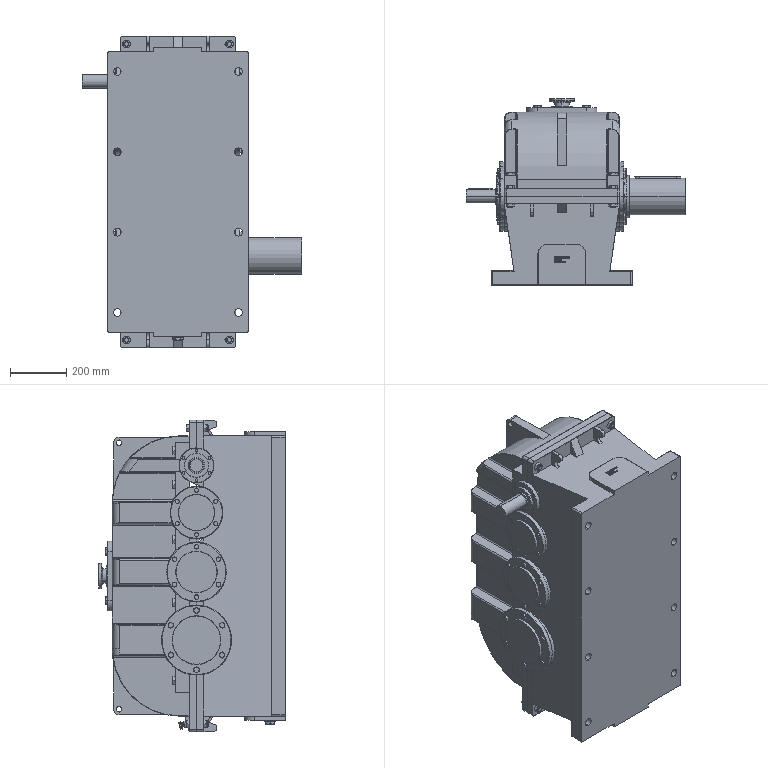Part | SolidWorks | features ICE 43, Extrusion 14, Fillet 9, CirPattern 5, Chamfer 4, MirrorPattern 4, DeleteBody 2, LPattern 1, RefAxis 1, Revolution 1 | 3 solids | 2648 faces | box 780 x 662 x 1105 mm | volume 238167448 mm3 | plane 1319 | cone 448 | spline 429 | cylinder 324 | torus 114 | sphere 14 | commonest cylinder face diameters 2 x108 9 x32 18 x16 28 x16 124 x12 186 x12